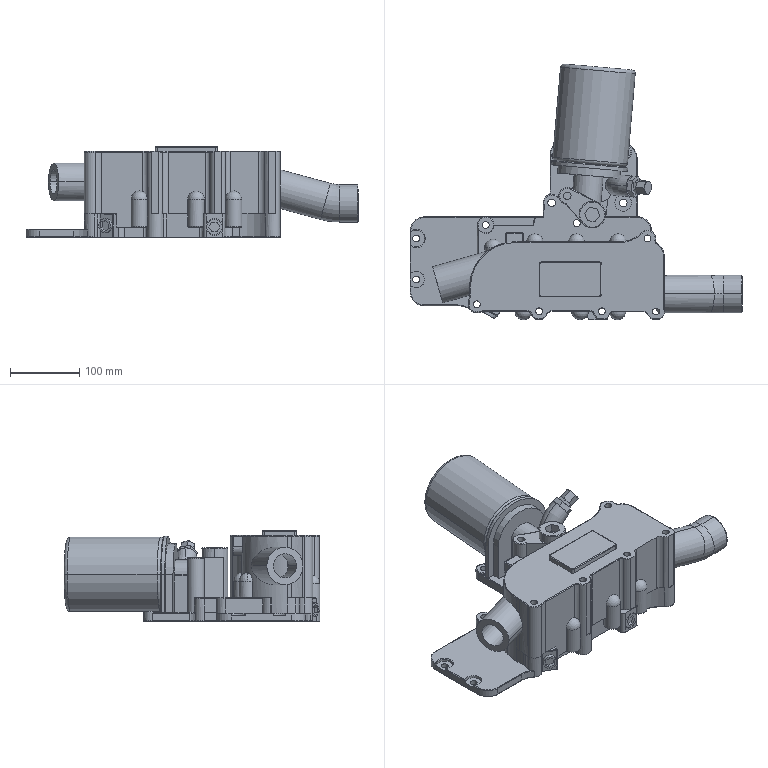Part | SolidWorks | features BaseBody 2 | 2 solids | 541 faces | box 478.032 x 368.283 x 131 mm | volume 5988897 mm3 | cylinder 249 | plane 189 | torus 79 | sphere 17 | spline 7 | commonest cylinder face diameters 2 x54 24 x35 10 x30 28 x17 24.5 x16 11 x10